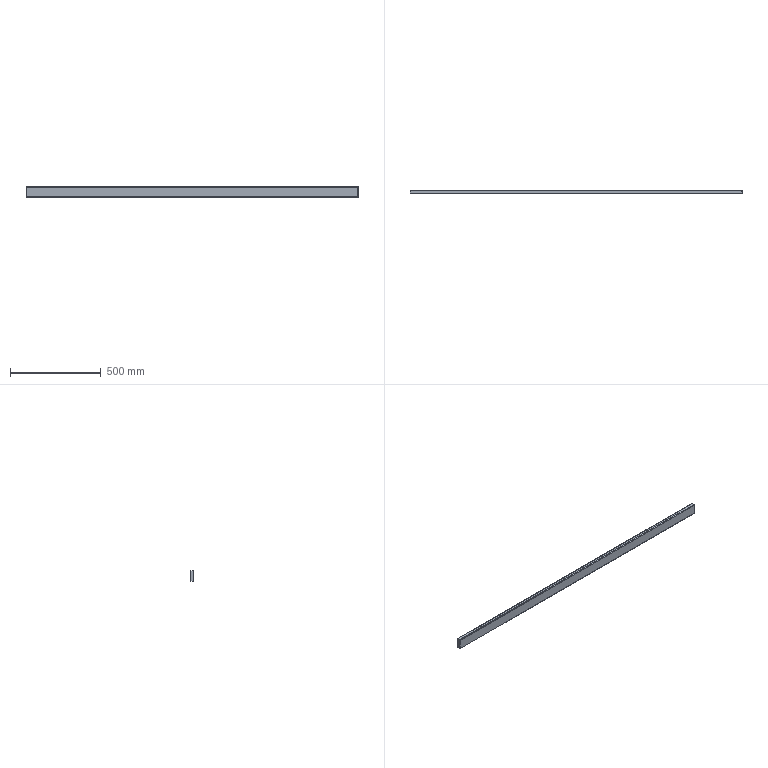Part | SolidWorks | features FlatPattern 6, SMBaseFlange 3, SheetMetal 3, EdgeFlange 2, HoleWzd 2, MirrorSolid 2, ICE 1, LPattern 1 | 8 solids | 98 faces | box 1828 x 20 x 60 mm | volume 338800 mm3 | plane 72 | cylinder 26 | commonest cylinder face diameters 7 x12 5 x10 4 x4